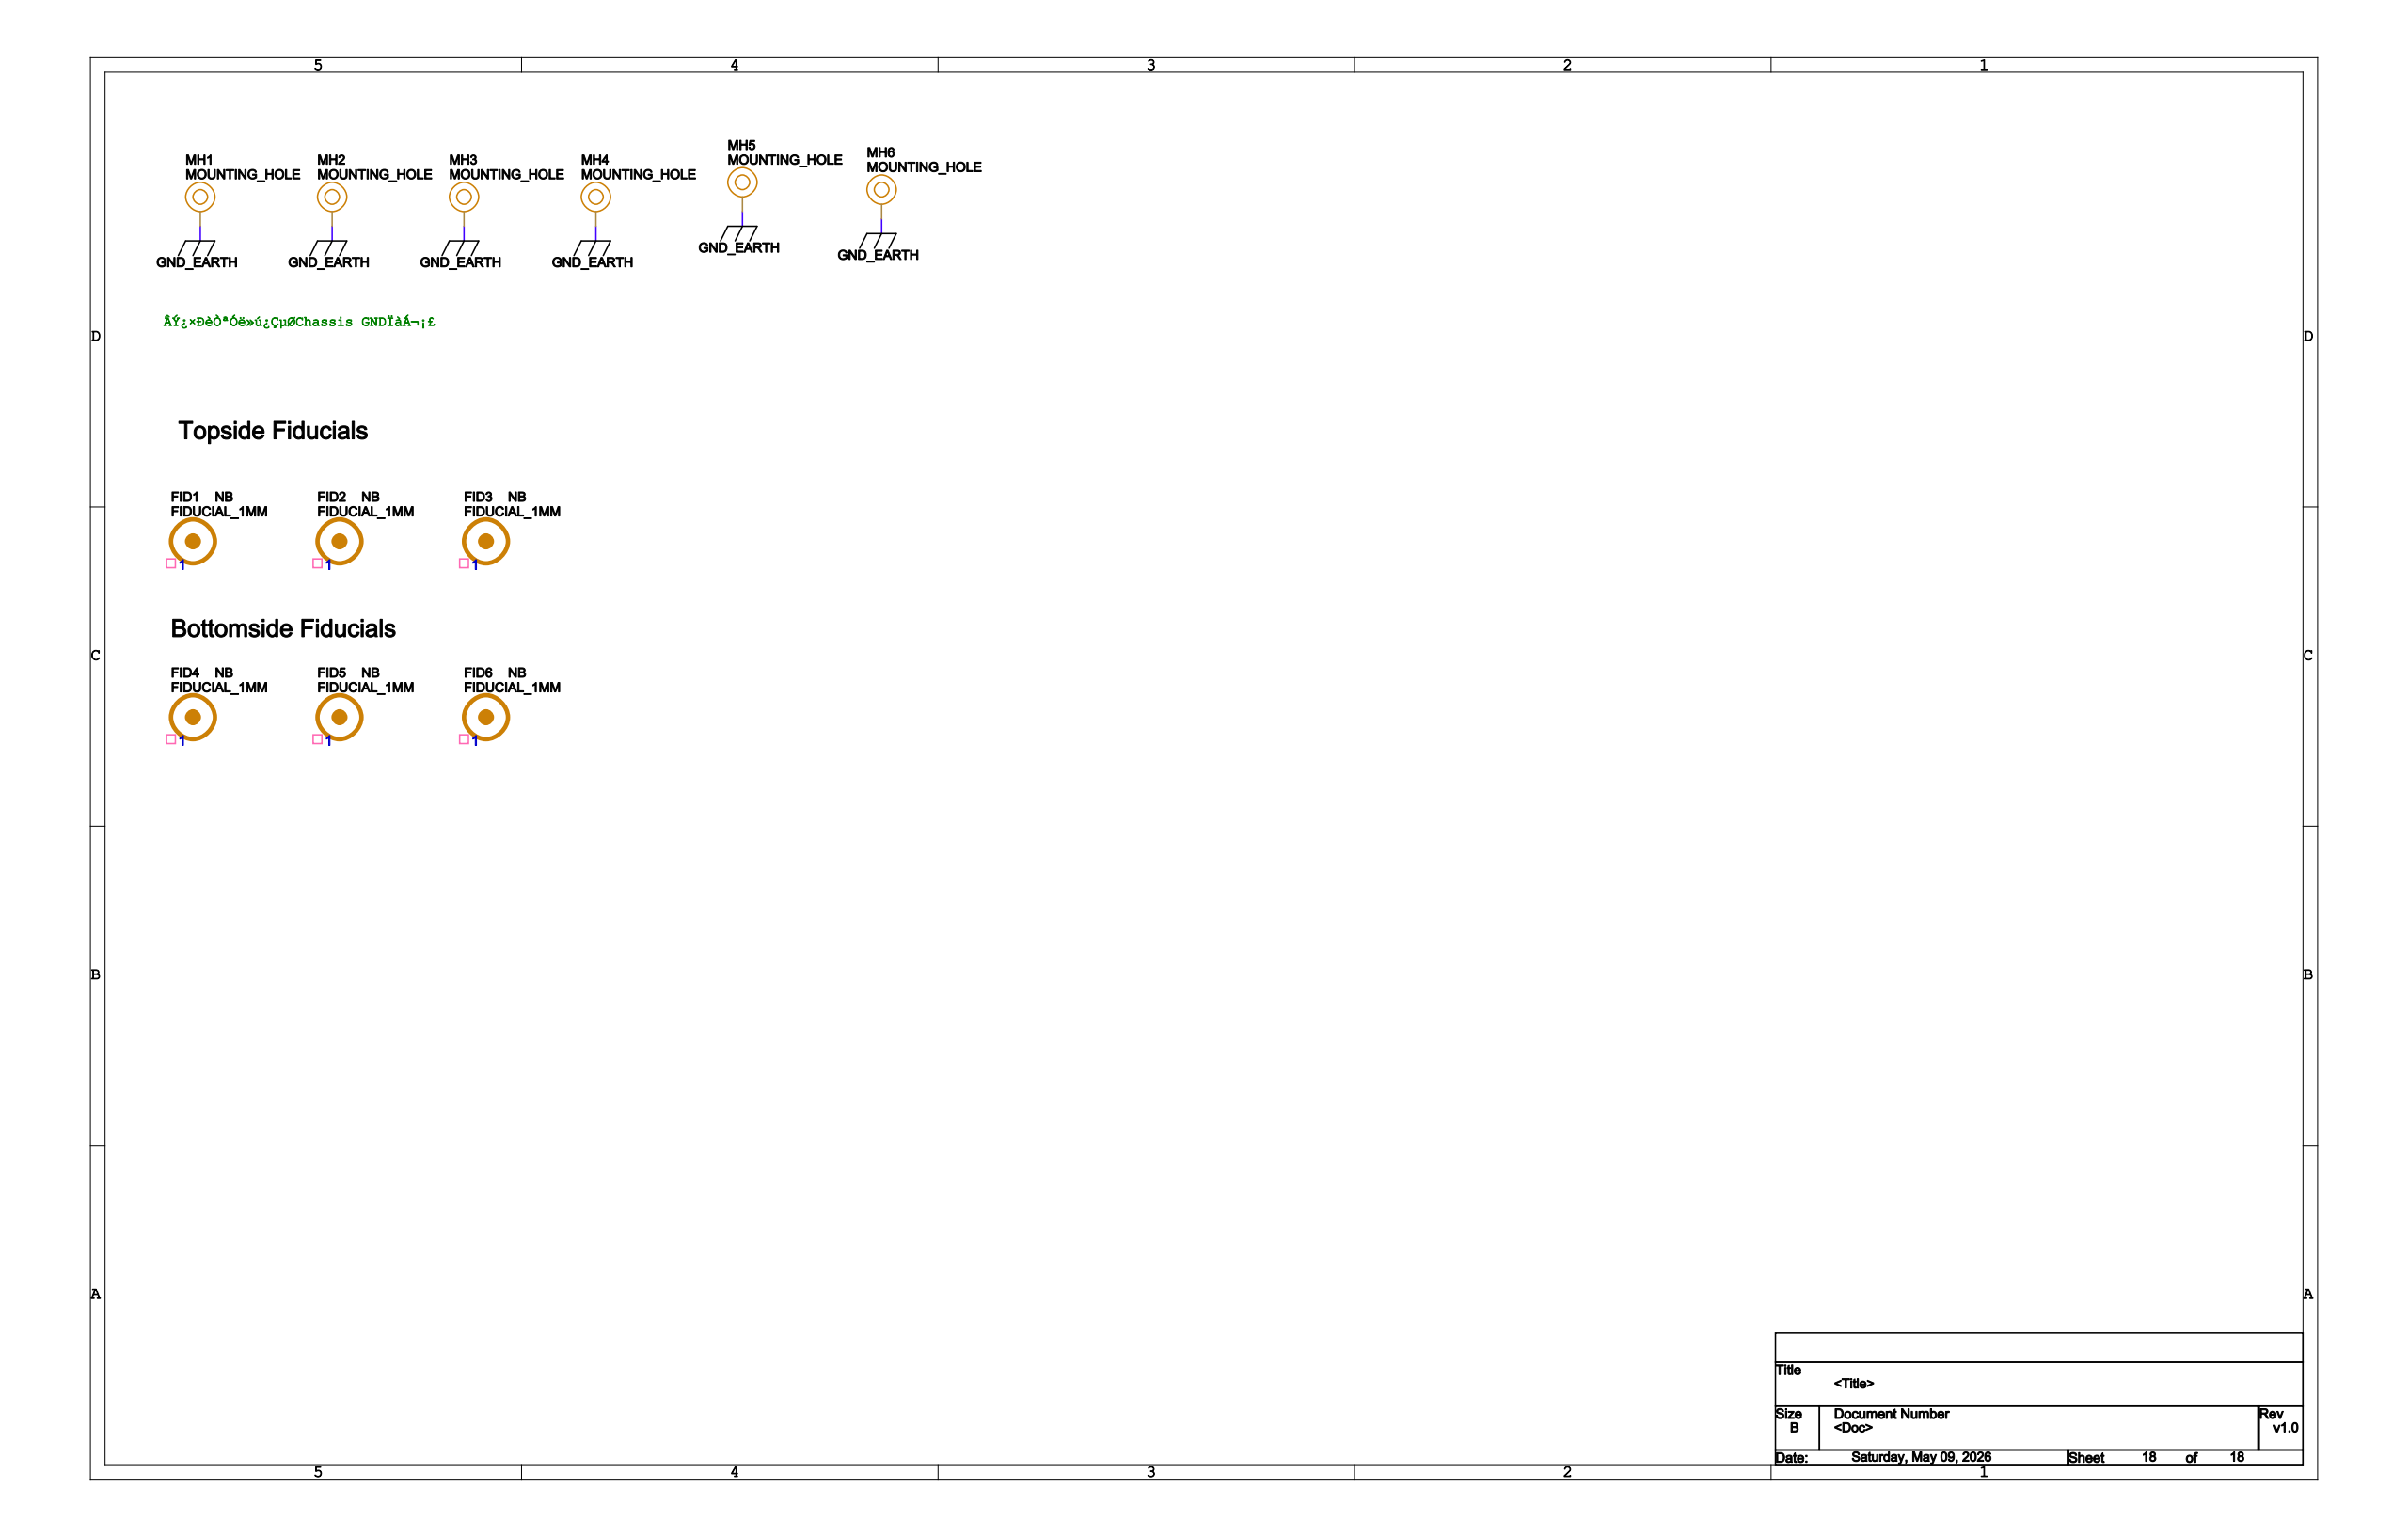Circuit board | Cadence Allegro | 330 parts | 215 nets | one sheet of the schematic
Parts on this sheet (reference | value | footprint):
MH1 | MOUNTING_HOLE | HOLE3_3MM_6
MH2 | MOUNTING_HOLE | HOLE3_3MM_6
MH3 | MOUNTING_HOLE | HOLE3_3MM_6
MH4 | MOUNTING_HOLE | HOLE3_3MM_6
MH5 | MOUNTING_HOLE | HOLE3_3MM_6
MH6 | MOUNTING_HOLE | HOLE3_3MM_6
Nets of these parts (net: part-pin ...):
GND_EARTH: MH1-1 MH2-1 MH3-1 MH4-1 MH5-1 MH6-1